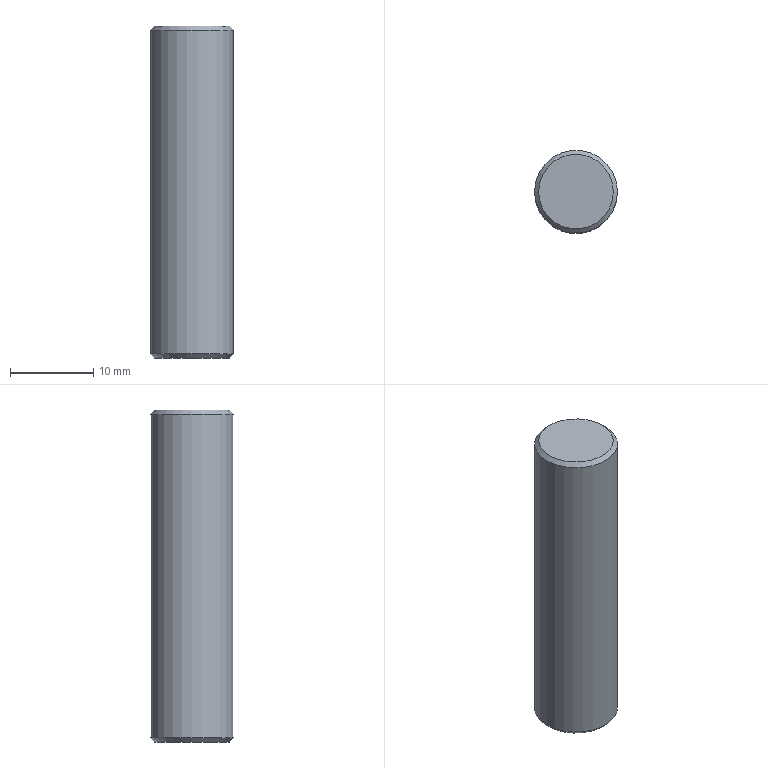Part | STEP file | D8-50_id78_x_t | 1 solid | 5 faces | box 10 x 10 x 40 mm | volume 3134 mm3 | plane 2 | cone 2 | cylinder 1 | commonest cylinder face diameters 10 x1
STEP:
#1=CARTESIAN_POINT('',(-287.,-69.5,-77.));
#2=VERTEX_POINT('',#1);
#3=CARTESIAN_POINT('',(-282.5,-69.5,-77.));
#4=DIRECTION('',(0.,0.,-1.));
#5=DIRECTION('',(-1.,0.,0.));
#6=AXIS2_PLACEMENT_3D('',#3,#4,#5);
#7=CIRCLE('',#6,4.5);
#8=EDGE_CURVE('',#2,#2,#7,.T.);
#9=ORIENTED_EDGE('',*,*,#8,.T.);
#10=EDGE_LOOP('',(#9));
#11=FACE_OUTER_BOUND('',#10,.T.);
#12=CARTESIAN_POINT('',(-282.5,-69.5,-77.));
#13=DIRECTION('',(0.,0.,-1.));
#14=DIRECTION('',(-1.,0.,0.));
#15=AXIS2_PLACEMENT_3D('',#12,#13,#14);
#16=PLANE('',#15);
#17=ADVANCED_FACE('',(#11),#16,.T.);
#18=CARTESIAN_POINT('',(-287.5,-69.5,-76.5));
#19=VERTEX_POINT('',#18);
#20=CARTESIAN_POINT('',(-282.5,-69.5,-76.5));
#21=DIRECTION('',(0.,0.,1.));
#22=DIRECTION('',(-1.,0.,0.));
#23=AXIS2_PLACEMENT_3D('',#20,#21,#22);
#24=CIRCLE('',#23,5.);
#25=EDGE_CURVE('',#19,#19,#24,.T.);
#26=ORIENTED_EDGE('',*,*,#25,.T.);
#27=EDGE_LOOP('',(#26));
#28=FACE_BOUND('',#27,.T.);
#29=CARTESIAN_POINT('',(-277.5,-69.5,-37.5));
#30=VERTEX_POINT('',#29);
#31=CARTESIAN_POINT('',(-282.5,-69.5,-37.5));
#32=DIRECTION('',(0.,0.,-1.));
#33=DIRECTION('',(1.,0.,0.));
#34=AXIS2_PLACEMENT_3D('',#31,#32,#33);
#35=CIRCLE('',#34,5.);
#36=EDGE_CURVE('',#30,#30,#35,.T.);
#37=ORIENTED_EDGE('',*,*,#36,.T.);
#38=EDGE_LOOP('',(#37));
#39=FACE_BOUND('',#38,.T.);
#40=CARTESIAN_POINT('',(-282.5,-69.5,-57.));
#41=DIRECTION('',(0.,0.,-1.));
#42=DIRECTION('',(1.,0.,0.));
#43=AXIS2_PLACEMENT_3D('',#40,#41,#42);
#44=CYLINDRICAL_SURFACE('',#43,5.);
#45=ADVANCED_FACE('',(#28,#39),#44,.T.);
#46=CARTESIAN_POINT('',(-278.,-69.5,-37.));
#47=VERTEX_POINT('',#46);
#48=CARTESIAN_POINT('',(-282.5,-69.5,-37.));
#49=DIRECTION('',(0.,0.,1.));
#50=DIRECTION('',(1.,0.,0.));
#51=AXIS2_PLACEMENT_3D('',#48,#49,#50);
#52=CIRCLE('',#51,4.5);
#53=EDGE_CURVE('',#47,#47,#52,.T.);
#54=ORIENTED_EDGE('',*,*,#53,.T.);
#55=EDGE_LOOP('',(#54));
#56=FACE_OUTER_BOUND('',#55,.T.);
#57=CARTESIAN_POINT('',(-282.5,-69.5,-37.));
#58=DIRECTION('',(0.,0.,1.));
#59=DIRECTION('',(1.,0.,0.));
#60=AXIS2_PLACEMENT_3D('',#57,#58,#59);
#61=PLANE('',#60);
#62=ADVANCED_FACE('',(#56),#61,.T.);
#63=ORIENTED_EDGE('',*,*,#8,.F.);
#64=EDGE_LOOP('',(#63));
#65=FACE_BOUND('',#64,.T.);
#66=ORIENTED_EDGE('',*,*,#25,.F.);
#67=EDGE_LOOP('',(#66));
#68=FACE_BOUND('',#67,.T.);
#69=CARTESIAN_POINT('',(-282.5,-69.5,-76.5));
#70=DIRECTION('',(0.,0.,1.));
#71=DIRECTION('',(1.,0.,0.));
#72=AXIS2_PLACEMENT_3D('',#69,#70,#71);
#73=CONICAL_SURFACE('',#72,5.,45.);
#74=ADVANCED_FACE('',(#65,#68),#73,.T.);
#75=ORIENTED_EDGE('',*,*,#53,.F.);
#76=EDGE_LOOP('',(#75));
#77=FACE_BOUND('',#76,.T.);
#78=ORIENTED_EDGE('',*,*,#36,.F.);
#79=EDGE_LOOP('',(#78));
#80=FACE_BOUND('',#79,.T.);
#81=CARTESIAN_POINT('',(-282.5,-69.5,-37.5));
#82=DIRECTION('',(0.,0.,-1.));
#83=DIRECTION('',(-1.,0.,0.));
#84=AXIS2_PLACEMENT_3D('',#81,#82,#83);
#85=CONICAL_SURFACE('',#84,5.,45.);
#86=ADVANCED_FACE('',(#77,#80),#85,.T.);
#87=CLOSED_SHELL('',(#17,#45,#62,#74,#86));
#88=MANIFOLD_SOLID_BREP('',#87);
#89=(LENGTH_UNIT()NAMED_UNIT(*)SI_UNIT(.MILLI.,.METRE.));
#90=UNCERTAINTY_MEASURE_WITH_UNIT(LENGTH_MEASURE(0.00002),#89,'','');
#91=(NAMED_UNIT(*)PLANE_ANGLE_UNIT()SI_UNIT($,.RADIAN.));
#92=PLANE_ANGLE_MEASURE_WITH_UNIT(PLANE_ANGLE_MEASURE(0.01745),#91);
#93=DIMENSIONAL_EXPONENTS(0.,0.,0.,0.,0.,0.,0.);
#94=(CONVERSION_BASED_UNIT('DEGREE',#92)NAMED_UNIT(#93)PLANE_ANGLE_UNIT());
#95=(NAMED_UNIT(*)SI_UNIT($,.STERADIAN.)SOLID_ANGLE_UNIT());
#96=(GEOMETRIC_REPRESENTATION_CONTEXT(3)GLOBAL_UNCERTAINTY_ASSIGNED_CONTEXT((#90))GLOBAL_UNIT_ASSIGNED_CONTEXT((#89,#94,#95))REPRESENTATION_CONTEXT('',''));
#97=ADVANCED_BREP_SHAPE_REPRESENTATION('',(#88),#96);